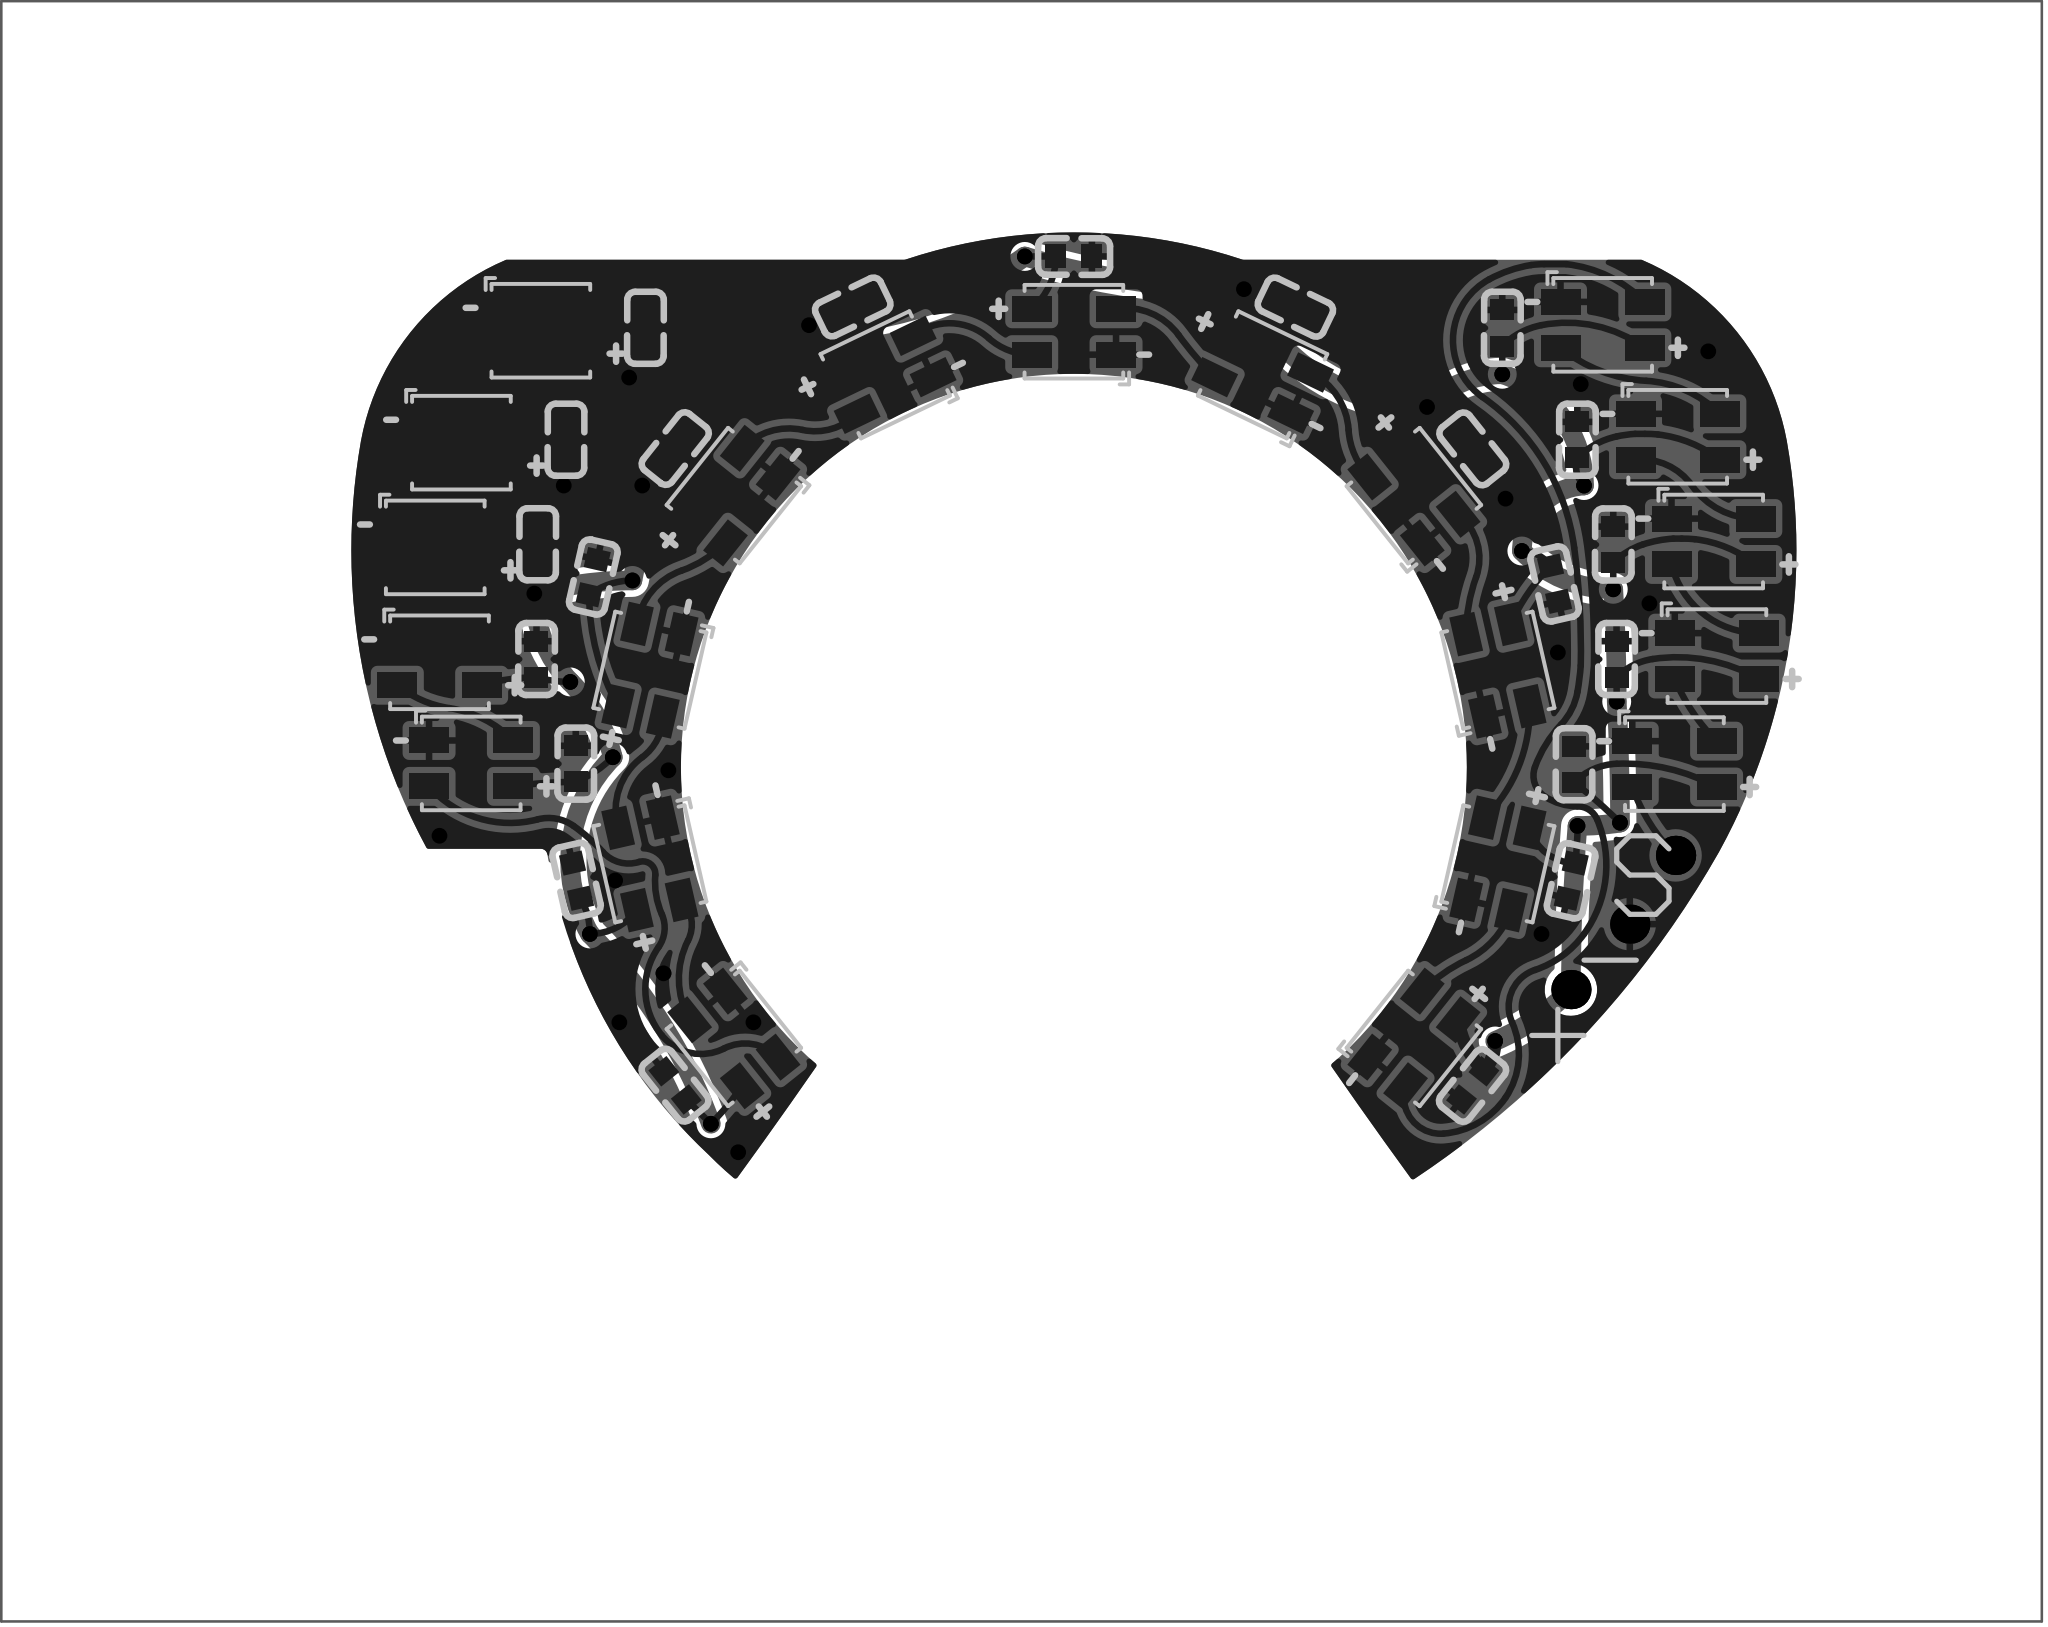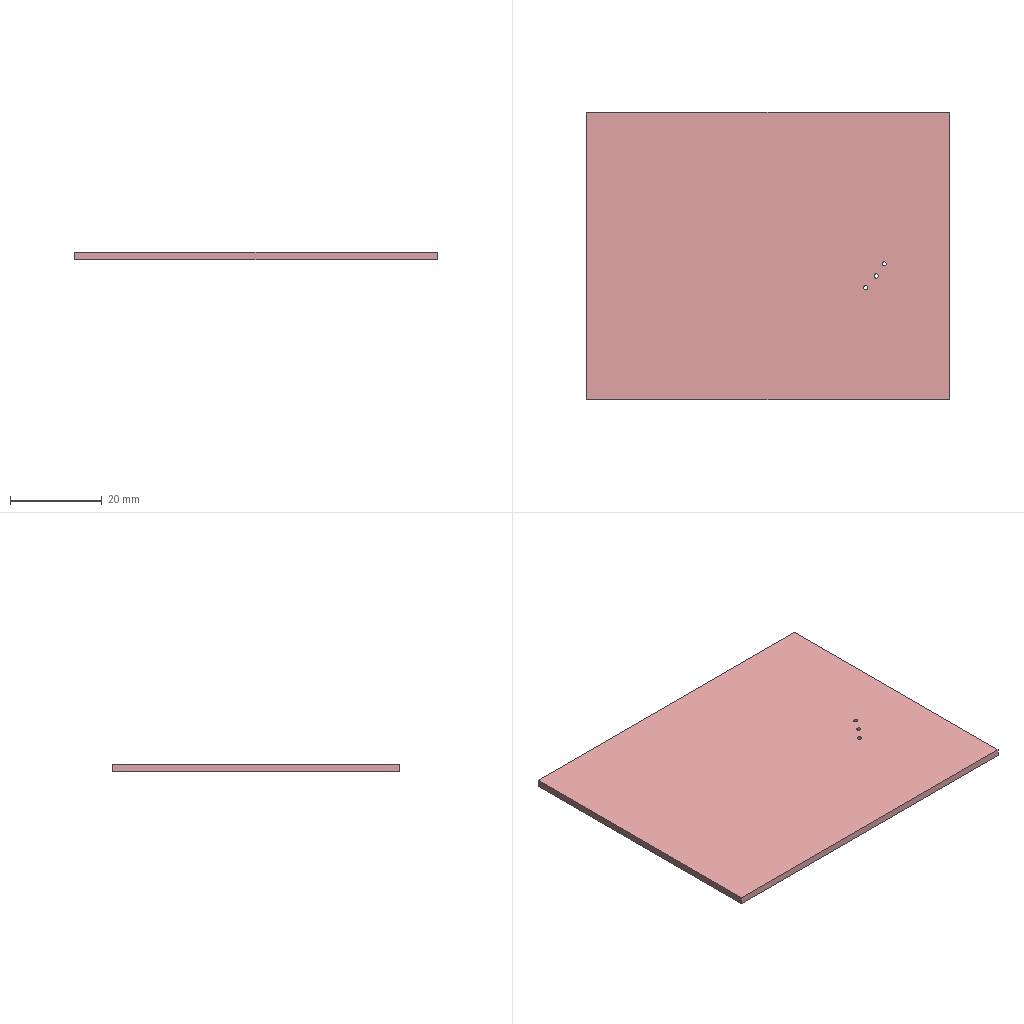Circuit board layout | Altium Designer | box 79.2 x 62.9 x 1.6 mm
Layer stack:
# Altium Designer layer stack of  (unit mm; dielectric type: 0 none, 1 core, 2 prepreg, 3 surface material)
index,name,kind,layer,copper_thickness_mm,dielectric_type,dielectric_thickness_mm,dielectric_material,dielectric_constant
0,Top Paste Mask Layer,other,,,,,,
1,Top Silkscreen Layer,other,,,,,,
2,Top Solder Mask Layer,dielectric,,,3,0.01,,3.3
3,Top Layer,copper,Top Layer,0.035,,,,
4,Dielectric1,dielectric,,,3,1.51,FR4,4.5
5,Bottom Layer,copper,Bottom Layer,0.035,,,,
6,Bottom Solder Mask Layer,dielectric,,,3,0.01,,3.3
7,Bottom Silkscreen Layer,other,,,,,,
8,Bottom Paste Mask Layer,other,,,,,,
# drill layer pairs: low layer,high layer
drill_pair,Top Layer,Bottom Layer
Part placement:
Designator,Comment,Layer,Footprint,Center-X(mm),Center-Y(mm),Rotation
LED1,WS2812B-Mini,TopLayer,LED-SMD_4P-L3.5-W3.5-TL_WS2812B,111.506,119.894,0
C1,100nF,TopLayer,C0603,111.506,122.815,180
LED1,WS2812B-Mini,TopLayer,LED-SMD_4P-L3.5-W3.5-TL_WS2812B,104.177,118.221,25.7
C1,100nF,TopLayer,C0603,102.91,120.853,205.7
LED1,WS2812B-Mini,TopLayer,LED-SMD_4P-L3.5-W3.5-TL_WS2812B,98.3,113.534,51.4
C1,100nF,TopLayer,C0603,96.016,115.355,231.4
LED1,WS2812B-Mini,TopLayer,LED-SMD_4P-L3.5-W3.5-TL_WS2812B,95.038,106.761,77.1
C1,100nF,TopLayer,C0603,92.837,110.369,257.1
LED1,WS2812B-Mini,TopLayer,LED-SMD_4P-L3.5-W3.5-TL_WS2812B,95.038,99.244,102.9
C1,100nF,TopLayer,C0603,92.191,98.594,282.9
LED1,WS2812B-Mini,TopLayer,LED-SMD_4P-L3.5-W3.5-TL_WS2812B,98.3,92.472,128.6
C1,100nF,TopLayer,C0603,96.016,90.65,308.6
LED1,WS2812B-Mini,TopLayer,LED-SMD_4P-L3.5-W3.5-TL_WS2812B,124.712,92.472,231.4
C1,100nF,TopLayer,C0603,126.996,90.65,51.4
LED1,WS2812B-Mini,TopLayer,LED-SMD_4P-L3.5-W3.5-TL_WS2812B,127.974,99.244,257.1
C1,100nF,TopLayer,C0603,130.821,98.594,77.1
LED1,WS2812B-Mini,TopLayer,LED-SMD_4P-L3.5-W3.5-TL_WS2812B,127.974,106.761,282.9
C1,100nF,TopLayer,C0603,130.175,110.115,102.9
LED1,WS2812B-Mini,TopLayer,LED-SMD_4P-L3.5-W3.5-TL_WS2812B,124.712,113.534,308.6
C1,100nF,TopLayer,C0603,126.996,115.355,128.6
LED1,WS2812B-Mini,TopLayer,LED-SMD_4P-L3.5-W3.5-TL_WS2812B,118.835,118.221,334.3
C1,100nF,TopLayer,C0603,120.102,120.853,154.3
LED1,WS2812B-Mini,TopLayer,LED-SMD_4P-L3.5-W3.5-TL_WS2812B,90.805,119.932,180
C1,100nF,TopLayer,C0603,94.864,120.038,270
LED1,WS2812B-Mini,TopLayer,LED-SMD_4P-L3.5-W3.5-TL_WS2812B,87.719,115.588,180
C1,100nF,TopLayer,C0603,91.778,115.695,270
LED1,WS2812B-Mini,TopLayer,LED-SMD_4P-L3.5-W3.5-TL_WS2812B,86.704,111.525,180
C1,100nF,TopLayer,C0603,90.678,111.639,270
LED1,WS2812B-Mini,TopLayer,LED-SMD_4P-L3.5-W3.5-TL_WS2812B,86.868,107.067,180
C1,100nF,TopLayer,C0603,90.635,107.186,270
LED1,WS2812B-Mini,TopLayer,LED-SMD_4P-L3.5-W3.5-TL_WS2812B,88.1,103.142,180
C1,100nF,TopLayer,C0603,92.159,103.127,270
LED1,WS2812B-Mini,TopLayer,LED-SMD_4P-L3.5-W3.5-TL_WS2812B,132.042,120.16,180
C1,100nF,TopLayer,C0603,128.143,120.038,270
LED1,WS2812B-Mini,TopLayer,LED-SMD_4P-L3.5-W3.5-TL_WS2812B,134.956,115.817,180
C1,100nF,TopLayer,C0603,131.057,115.695,270
LED1,WS2812B-Mini,TopLayer,LED-SMD_4P-L3.5-W3.5-TL_WS2812B,136.353,111.753,180
C1,100nF,TopLayer,C0603,132.454,111.631,270
LED1,WS2812B-Mini,TopLayer,LED-SMD_4P-L3.5-W3.5-TL_WS2812B,136.48,107.308,180
C1,100nF,TopLayer,C0603,132.581,107.186,270
LED1,WS2812B-Mini,TopLayer,LED-SMD_4P-L3.5-W3.5-TL_WS2812B,134.829,103.117,180
C1,100nF,TopLayer,C0603,130.93,103.104,270
Pad and via stacks:
# Altium Designer via and pad stacks of  (unit mm). Each distinct definition once, with the count of objects using it.
# via: kind,start_layer,end_layer,hole_mm,diameter_mm,mode(0 simple;1 top-mid-bottom;2 full stack),diameter_per_layer,count,example_net
# pad: kind,layer,hole_mm,hole_type(0 round;1 square;2 slot),plating,top_size,top_shape(1 round;2 rect;3 octagon;9 rounded rect),mid_size,bottom_size,mode,footprint,size_per_layer,count,example
pad,Multi-Layer,0.9144,0,plated,1.524x1.524,1,1.524x1.524,1.524x1.524,0,,,3,1
pad,Top Layer,0,0,plated,1.545x0.997,2,1.545x0.997,1.545x0.997,0,LED-SMD_4P-L3.5-W3.5-TL_WS2812B,,84,LED1.1
pad,Top Layer,0,0,plated,0.8x0.9,2,0.8x0.9,0.8x0.9,0,C0603,,42,C1.2
via,Top Layer,Bottom Layer,0.3048,0.61,0,,34,VCC
Copper pours:
name,layer,net,type(0 solid;1 hatched;2 none)
Bottom Layer-GND,Bottom Layer,GND,0
Top Layer-GND,Top Layer,GND,0